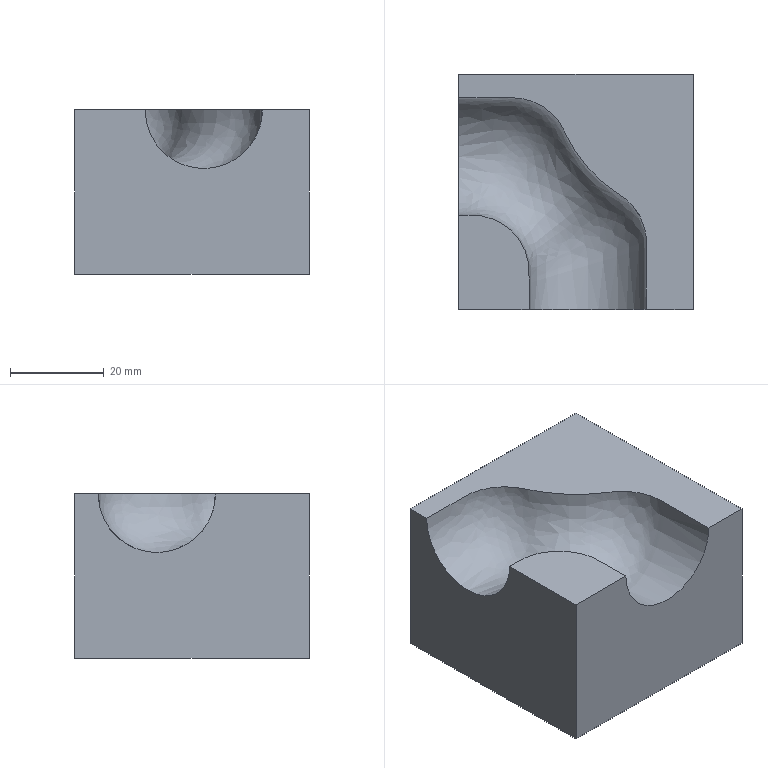NC program | NX | posted with a generic post | part box 50 x 50 x 35 mm
Lines 1 to 1307 of 32931:
N10 G17 G21 G94 G90
(CAVITY_MILL , TOOL : D12)
N12 T00 M6
N14 G54
N16 G17 G0 G90 X-6. Y32.437 S3000 M3
N18 G43 Z10. H0
N20 Z-0.097
N22 G94 G1 Z-0.297 F2500.
N24 X5.4
N26 Y31.532
N28 G2 X14.08 Y28.901 R23.645
N30 X11.92 Y33.111 R41.565
N32 G3 X11.609 Y33.334 R0.377
N34 G1 X9.998 Y33.341
N36 X5.4 Y33.342
N38 Y32.437
N40 X0.
N42 Y26.25
N44 X3.16 Y26.252
N46 G2 X19.984 Y14.699 R18.245
N48 G1 X25.008 Y16.679
N50 G2 X26.652 Y8.373 R23.645
N52 G1 X26.662 Y7.474
N54 X26.663 Y5.4
N56 X28.34
N58 Y14.217
N60 G3 X28.198 Y14.478 R0.312
N62 G2 X26.484 Y15.623 R100.713
N64 X25.008 Y16.679 R41.565
N66 G1 X19.984 Y14.699
N68 G2 X21.252 Y8.298 R18.245
N70 G1 X21.262 Y7.442
N72 X21.264 Y0.591
N74 X21.256 Y0.
N76 X33.748
N78 X33.741 Y0.591
N80 X33.74 Y14.217
N82 G3 X31.151 Y18.999 R5.712
N84 G2 X29.529 Y20.082 R95.313
N86 X16.858 Y35.298 R36.165
N88 G3 X11.724 Y38.733 R5.777
N90 G1 X10.011 Y38.741
N92 X0. Y38.743
N94 Y32.437
N96 X-6.
N98 Z-0.097
N100 G0 Z0.3
N102 Y32.434
N104 Z-0.395
N106 G1 Z-0.595
N108 X5.4
N110 Y31.545
N112 G2 X14.054 Y28.93 R23.661
N114 X12.004 Y32.909 R41.601
N116 G3 X11.822 Y33.205 R3.769
N118 X11.607 Y33.319 R0.261
N120 G1 X5.4 Y33.324
N122 Y32.434
N124 X0.
N126 Y26.261
N128 X3.16 Y26.265
N130 G2 X20.015 Y14.66 R18.261
N132 G1 X25.043 Y16.627
N134 G2 X26.668 Y8.366 R23.661
N136 G1 X26.676 Y7.467
N138 Y5.4
N140 X28.33
N142 Y13.425
N144 X28.327 Y14.197
N146 G3 X28.174 Y14.479 R0.339
N148 G1 X26.712 Y15.443
N150 G2 X25.043 Y16.627 R41.601
N152 G1 X20.015 Y14.66
N154 G2 X21.268 Y8.298 R18.261
N156 G1 X21.276 Y7.442
N158 X21.278 Y0.591
N160 X21.272 Y0.
N162 X33.736
N164 X33.73 Y0.591
N166 Y13.436
N168 X33.727 Y14.22
N170 G3 X31.145 Y18.988 R5.739
N172 G1 X29.708 Y19.935
N174 G2 X16.862 Y35.274 R36.201
N176 G3 X16.287 Y36.242 R9.169
N178 X11.611 Y38.719 R5.661
N180 G1 X0. Y38.728
N182 Y32.434
N184 X-6.
N186 Z-0.395
N188 G0 Z0.003
N190 Z-0.692
N192 G1 Z-0.892
N194 X5.4
N196 Y31.56
N198 G2 X13.994 Y28.981 R23.668
N200 X11.935 Y33. R41.381
N202 G3 X11.767 Y33.244 R0.8
N204 G1 X11.69 Y33.312
N206 X11.588 Y33.305
N208 X5.4 Y33.309
N210 Y32.434
N212 X0.
N214 Y26.282
N216 X3.16 Y26.28
N218 G2 X20.04 Y14.642 R18.268
N220 G1 X25.072 Y16.602
N222 G2 X26.683 Y8.357 R23.668
N224 G1 X26.689 Y7.46
N226 X26.69 Y5.4
N228 X28.315
N230 X28.316 Y13.405
N232 X28.307 Y14.195
N234 G3 X28.153 Y14.479 R0.347
N236 G1 X26.693 Y15.458
N238 G2 X25.072 Y16.602 R41.381
N240 G1 X20.04 Y14.642
N242 G2 X21.284 Y8.298 R18.268
N244 G1 X21.289 Y7.442
N246 X21.292 Y0.591
N248 X21.288 Y0.
N250 X33.72
N252 X33.714 Y0.591
N254 X33.716 Y13.436
N256 X33.706 Y14.258
N258 G3 X31.161 Y18.964 R5.747
N260 G1 X29.701 Y19.943
N262 G2 X16.869 Y35.196 R35.981
N264 G3 X15.149 Y37.458 R6.2
N266 X11.724 Y38.704 R5.846
N268 G1 X0. Y38.713
N270 Y32.434
N272 X-6.
N274 Z-0.692
N276 G0 Z-0.295
N278 Y32.436
N280 Z-0.989
N282 G1 Z-1.189
N284 X5.4
N286 Y31.583
N288 G2 X13.921 Y29.049 R23.678
N290 X11.883 Y33.058 R41.348
N292 G3 X11.573 Y33.28 R0.375
N294 G1 X10.835 Y33.289
N296 X5.4 Y33.288
N298 Y32.436
N300 X0.
N302 Y26.31
N304 X3.16 Y26.316
N306 X3.887 Y26.282
N308 G2 X20.095 Y14.572 R18.278
N310 G1 X25.136 Y16.506
N312 G2 X26.42 Y11.707 R23.678
N314 X26.699 Y8.163 R22.996
N316 G1 X26.703 Y5.4
N318 X28.288
N320 X28.291 Y13.412
N322 X28.283 Y14.218
N324 X28.291 Y14.323
N326 X28.213 Y14.393
N328 X26.709 Y15.4
N330 G2 X25.136 Y16.506 R41.348
N332 G1 X20.095 Y14.572
N334 G2 X21.085 Y10.867 R18.278
N336 X21.299 Y8.155 R17.596
N338 G1 X21.31 Y0.591
N340 X21.305 Y0.
N342 X33.691
N344 X33.687 Y0.591
N346 X33.691 Y13.436
N348 X33.683 Y14.293
N350 G3 X31.42 Y18.745 R5.677
N352 G1 X29.713 Y19.888
N354 G2 X16.822 Y35.24 R35.948
N356 G3 X11.724 Y38.679 R5.775
N358 G1 X10.867 Y38.689
N360 X0.591 Y38.687
N362 X0. Y38.692
N364 Y32.436
N366 X-6.
N368 Z-0.989
N370 G0 Z-0.592
N372 Y32.433
N374 Z-1.287
N376 G1 Z-1.487
N378 X5.4
N380 Y31.62
N382 G2 X13.839 Y29.121 R23.937
N384 X11.854 Y33.065 R41.036
N386 G3 X11.599 Y33.247 R0.307
N388 G1 X10.847 Y33.254
N390 X5.4 Y33.247
N392 Y32.433
N394 X0.
N396 Y26.351
N398 G2 X3.49 Y26.339 R66.439
N400 X16.647 Y20.287 R18.537
N402 X20.169 Y14.496 R18.185
N404 G1 X25.225 Y16.393
N406 G2 X26.726 Y8.333 R23.585
N408 G1 X26.733 Y5.4
N410 X28.258
N412 X28.254 Y14.231
N414 X28.26 Y14.327
N416 X28.178 Y14.376
N418 G3 X27.166 Y15.057 R33.566
N420 G2 X25.225 Y16.393 R41.036
N422 G1 X20.169 Y14.496
N424 G2 X21.326 Y8.298 R18.185
N426 G1 X21.345 Y0.591
N428 X21.341 Y0.
N430 X33.661
N432 X33.654 Y14.234
N434 G3 X31.273 Y18.802 R5.578
N436 X30.098 Y19.591 R38.966
N438 G2 X16.801 Y35.23 R35.636
N440 G3 X11.724 Y38.647 R5.707
N442 G1 X10.867 Y38.654
N444 X1.447 Y38.641
N446 X0. Y38.648
N448 Y32.433
N450 X-6.
N452 Z-1.287
N454 G0 Z-0.889
N456 Z-1.584
N458 G1 Z-1.784
N460 X5.4
N462 Y31.661
N464 G2 X13.742 Y29.214 R24.5
N466 X11.836 Y33.019 R41.039
N468 G3 X11.537 Y33.214 R0.325
N470 G1 X5.4 Y33.204
N472 Y32.433
N474 X0.
N476 Y26.385
N478 G2 X3.16 Y26.397 R111.809
N480 X11.724 Y24.18 R19.1
N482 X20.247 Y14.407 R18.153
N484 G1 X25.316 Y16.268
N486 G2 X26.759 Y8.332 R23.553
N488 G1 X26.771 Y5.4
N490 X28.217
N492 X28.214 Y14.23
N494 X28.224 Y14.311
N496 X28.151 Y14.35
N498 G3 X27.438 Y14.826 R20.331
N500 G2 X25.316 Y16.268 R41.039
N502 G1 X20.247 Y14.407
N504 G2 X21.359 Y8.298 R18.153
N506 G1 X21.391 Y0.591
N508 X21.386 Y0.
N510 X33.618
N512 X33.614 Y14.231
N514 G3 X31.243 Y18.777 R5.547
N516 X30.34 Y19.38 R25.731
N518 G1 X30.277 Y19.42
N520 G2 X16.783 Y35.185 R35.639
N522 G3 X11.528 Y38.614 R5.725
N524 G1 X1.447 Y38.598
N526 X0. Y38.603
N528 Y32.433
N530 X-6.
N532 Z-1.584
N534 G0 Z-1.187
N536 Y32.436
N538 Z-1.881
N540 G1 Z-2.081
N542 X5.4
N544 Y31.71
N546 G2 X13.63 Y29.321 R24.108
N548 X11.814 Y32.976 R40.78
N550 G3 X11.509 Y33.176 R0.332
N552 G1 X5.4 Y33.162
N554 Y32.436
N556 X0.
N558 Y26.428
N560 X3.16 Y26.438
N562 G2 X17.718 Y19.154 R18.708
N564 X20.326 Y14.319 R18.41
N566 G1 X25.408 Y16.145
N568 G2 X26.81 Y8.34 R23.81
N570 G1 X26.823 Y5.4
N572 X28.174
N574 X28.183 Y13.413
N576 X28.175 Y14.206
N578 X28.184 Y14.288
N580 X28.11 Y14.326
N582 X27.592 Y14.677
N584 X27.274 Y14.881
N586 G2 X25.408 Y16.145 R40.78
N588 G1 X20.326 Y14.319
N590 G2 X21.41 Y8.298 R18.41
N592 G1 X21.444 Y0.591
N594 X21.44 Y0.
N596 X33.573
N598 X33.57 Y0.591
N600 X33.583 Y13.436
N602 X33.575 Y14.258
N604 G3 X31.14 Y18.796 R5.547
N606 G1 X30.564 Y19.187
N608 X30.182 Y19.431
N610 G2 X16.765 Y35.133 R35.38
N612 G3 X11.497 Y38.576 R5.732
N614 G1 X1.447 Y38.554
N616 X0. Y38.558
N618 Y32.436
N620 X-6.
N622 Z-1.881
N624 G0 Z-1.484
N626 Y32.435
N628 Z-2.179
N630 G1 Z-2.379
N632 X5.4
N634 Y31.754
N636 G2 X13.496 Y29.448 R24.115
N638 X11.946 Y32.57 R40.388
N640 G1 X11.727 Y33.02
N642 G3 X11.56 Y33.124 R0.185
N644 G1 X5.4 Y33.115
N646 Y32.435
N648 X0.
N650 Y26.48
N652 X3.16 Y26.479
N654 G2 X17.718 Y19.251 R18.715
N656 X20.423 Y14.21 R18.473
N658 G1 X25.519 Y15.995
N660 G2 X26.861 Y8.342 R23.873
N662 G1 X26.877 Y5.4
N664 X28.118
N666 X28.132 Y13.407
N668 X28.122 Y14.212
N670 X28.136 Y14.27
N672 X28.079 Y14.29
N674 X27.603 Y14.605
N676 X27.166 Y14.888
N678 G2 X25.519 Y15.995 R40.388
N680 G1 X20.423 Y14.21
N682 G2 X21.461 Y8.298 R18.473
N684 G1 X21.498 Y1.447
N686 X21.493 Y0.
N688 X33.514
N690 X33.509 Y0.591
N692 X33.532 Y13.436
N694 X33.521 Y14.281
N696 G3 X31.06 Y18.792 R5.495
N698 G1 X30.564 Y19.121
N700 X30.086 Y19.431
N702 G2 X16.844 Y34.846 R34.988
N704 G1 X16.581 Y35.385
N706 G3 X11.553 Y38.524 R5.585
N708 G1 X1.447 Y38.51
N710 X0. Y38.513
N712 Y32.435
N714 X-6.
N716 Z-2.179
N718 G0 Z-1.781
N720 Y32.433
N722 Z-2.476
N724 G1 Z-2.676
N726 X5.4
N728 Y31.806
N730 G2 X13.345 Y29.587 R24.307
N732 X11.727 Y32.92 R40.275
N734 G3 X11.504 Y33.066 R0.243
N736 G1 X5.4 Y33.059
N738 Y32.433
N740 X0.
N742 Y26.549
N744 G2 X3.368 Y26.527 R100.562
N746 X16.862 Y20.406 R18.907
N748 X20.53 Y14.087 R18.513
N750 G1 X25.643 Y15.823
N752 G2 X26.912 Y8.335 R23.913
N754 G1 X26.926 Y5.4
N756 X28.054
N758 X28.07 Y13.411
N760 X28.061 Y14.211
N762 X28.076 Y14.243
N764 X28.041 Y14.249
N766 X27.645 Y14.511
N768 X27.079 Y14.863
N770 G2 X25.643 Y15.823 R40.275
N772 G1 X20.53 Y14.087
N774 G2 X21.512 Y8.298 R18.513
N776 G1 X21.55 Y0.591
N778 X21.548 Y0.
N780 X33.448
N782 X33.444 Y0.591
N784 X33.47 Y13.436
N786 X33.461 Y14.272
N788 G3 X31.023 Y18.75 R5.445
N790 G1 X30.564 Y19.055
N792 X29.96 Y19.431
N794 G2 X16.689 Y35.052 R34.875
N796 G3 X11.498 Y38.466 R5.643
N798 G1 X0.591 Y38.453
N800 X0. Y38.457
N802 Y32.433
N804 X-6.
N806 Z-2.476
N808 G0 Z-2.079
N810 Y32.434
N812 Z-2.773
N814 G1 Z-2.973
N816 X5.4
N818 Y31.879
N820 G2 X13.196 Y29.73 R24.609
N822 X11.669 Y32.904 R40.408
N824 G1 X11.629 Y32.996
N826 X11.53
N828 X5.4 Y32.989
N830 Y32.434
N832 X0.
N834 Y26.617
N836 X0.01
N838 X3.16 Y26.609
N840 G2 X16.006 Y21.397 R19.209
N842 X20.646 Y13.974 R17.982
N844 G1 X25.784 Y15.636
N846 G2 X26.695 Y11.67 R23.382
N848 X26.963 Y8.313 R21.11
N850 G1 X26.98 Y5.4
N852 X27.991
N854 X28.009 Y13.416
N856 X28.002 Y14.175
N858 X28.008 Y14.242
N860 X27.944 Y14.262
N862 X27.842 Y14.318
N864 X26.971 Y14.852
N866 G2 X25.784 Y15.636 R39.985
N868 G1 X20.646 Y13.974
N870 G2 X21.355 Y10.867 R17.982
N872 X21.563 Y8.298 R15.71
N874 G1 X21.613 Y0.02
N876 Y0.
N878 X33.383
N880 X33.38 Y0.591
N882 X33.409 Y13.436
N884 X33.401 Y14.293
N886 G3 X30.564 Y18.983 R5.513
N888 G1 X29.833 Y19.431
N890 G2 X22.745 Y25.426 R34.585
N892 G1 X22.023 Y26.282
N894 G2 X16.632 Y35.031 R35.008
N896 G3 X11.524 Y38.396 R5.551
N898 G1 X0. Y38.384
N900 Y32.434
N902 X-6.
N904 Z-2.773
N906 G0 Z-2.376
N908 Z-3.071
N910 G1 Z-3.271
N912 X5.4
N914 Y31.952
N916 G2 X13.019 Y29.895 R24.659
N918 X11.626 Y32.851 R39.555
N920 G1 X11.598 Y32.93
N922 X11.515 Y32.925
N924 X5.4 Y32.916
N926 Y32.434
N928 X0.
N930 Y26.689
N932 X3.16 Y26.681
N934 G2 X16.862 Y20.652 R19.259
N936 X20.783 Y13.822 R18.257
N938 G1 X25.936 Y15.438
N940 G2 X26.998 Y9.37 R23.657
N942 G1 X27.033 Y8.419
N944 X27.058 Y5.4
N946 X27.92
N948 X27.938 Y14.148
N950 X27.948 Y14.193
N952 X27.902 Y14.194
N954 X27.848 Y14.225
N956 G2 X25.936 Y15.438 R39.555
N958 G1 X20.783 Y13.822
N960 G2 X21.602 Y9.155 R18.257
N962 G1 X21.633 Y8.298
N964 X21.697 Y0.591
N966 X21.695 Y0.
N968 X33.31
N970 Y0.002
N972 X33.338 Y14.293
N974 G3 X30.564 Y18.892 R5.477
N976 G2 X16.602 Y34.949 R34.155
N978 G3 X11.507 Y38.325 R5.521
N980 G1 X0. Y38.309
N982 Y32.434
N984 X-6.
N986 Z-3.071
N988 G0 Z-2.673
N990 Y32.435 Z-3.368
N992 G1 Z-3.568
N994 X5.4
N996 Y32.036
N998 G2 X12.829 Y30.069 R24.969
N1000 X11.562 Y32.8 R39.199
N1002 G1 X11.551 Y32.859
N1004 X11.492 Y32.847
N1006 X5.4 Y32.833
N1008 Y32.435
N1010 X0.
N1012 Y26.781
N1014 X3.16 Y26.769
N1016 G2 X15.605 Y22. R19.569
N1018 X20.912 Y13.708 R17.587
N1020 G1 X26.093 Y15.23
N1022 G2 X26.491 Y13.679 R22.987
N1024 G1 X26.691 Y12.643
N1026 G2 X27.099 Y8.814 R22.848
N1028 G1 X27.108 Y8.381
N1030 X27.134 Y5.4
N1032 X27.835
N1034 X27.855 Y14.13
N1036 X27.846 Y14.135
N1038 G2 X26.093 Y15.23 R39.199
N1040 G1 X20.912 Y13.708
N1042 G2 X21.203 Y12.58 R17.587
N1044 G1 X21.388 Y11.621
N1046 G2 X21.7 Y8.696 R17.448
N1048 G1 X21.709 Y8.298
N1050 X21.776 Y0.591
N1052 X21.774 Y0.
N1054 X33.222
N1056 Y0.006
N1058 X33.255 Y14.293
N1060 G3 X30.564 Y18.802 R5.374
N1062 G2 X16.544 Y34.883 R33.799
N1064 G3 X11.48 Y38.247 R5.476
N1066 G1 X0.007 Y38.22
N1068 X0.
N1070 Y32.435
N1072 X-6.
N1074 Z-3.368
N1076 G0 Z-2.971
N1078 Y32.432
N1080 Z-3.665
N1082 G1 Z-3.865
N1084 X5.4
N1086 Y32.133
N1088 G2 X12.636 Y30.252 R25.239
N1090 X11.498 Y32.749 R38.881
N1092 G1 X5.4 Y32.732
N1094 Y32.432
N1096 X0.
N1098 Y26.882
N1100 X0.032
N1102 X3.16 Y26.869
N1104 G2 X16.006 Y21.785 R19.839
N1106 X20.842 Y14.293 R17.777
N1108 X21.044 Y13.594 R22.457
N1110 G1 X26.256 Y15.004
N1112 G2 X27.176 Y9.356 R27.857
N1114 G1 X27.219 Y5.4
N1116 X27.749
N1118 X27.772 Y14.069
N1120 G2 X26.256 Y15.004 R38.881
N1122 G1 X21.044 Y13.594
N1124 G2 X21.777 Y9.155 R22.457
N1126 G1 X21.872 Y0.591
N1128 X21.87 Y0.
N1130 X33.135
N1132 X33.172 Y14.106
N1134 G3 X30.54 Y18.706 R5.31
N1136 G2 X16.482 Y34.828 R33.481
N1138 G3 X11.502 Y38.149 R5.372
N1140 G1 X0.047 Y38.118
N1142 X0.
N1144 Y32.432
N1146 X-6.
N1148 Z-3.665
N1150 G0 Z-3.268
N1152 Y32.43
N1154 Z-3.963
N1156 G1 Z-4.163
N1158 X5.4
N1160 Y32.229
N1162 G2 X12.439 Y30.44 R25.453
N1164 X11.438 Y32.65 R35.685
N1166 G1 X5.4 Y32.632
N1168 Y32.43
N1170 X0.
N1172 Y26.982
N1174 X0.038
N1176 X2.802 Y26.971
N1178 G2 X15.932 Y22. R20.053
N1180 X20.64 Y15.149 R17.441
N1182 G1 X20.956 Y14.293
N1184 G3 X21.153 Y13.54 R20.986
N1186 G1 X21.202 Y13.362
N1188 X26.413 Y14.776
N1190 G2 X27.27 Y8.689 R24.635
N1192 G1 X27.3 Y6.657
N1194 X27.315 Y5.4
N1196 X27.637
N1198 X27.676 Y14.01
N1200 G2 X26.413 Y14.776 R38.182
N1202 G1 X21.202 Y13.362
N1204 G2 X21.871 Y8.609 R19.235
N1206 G1 X21.901 Y6.585
N1208 X21.971 Y0.591
N1210 X21.969 Y0.
N1212 X33.019
N1214 X33.015 Y0.591
N1216 X33.077 Y14.293
N1218 G3 X30.564 Y18.578 R5.215
N1220 G2 X17.718 Y31.983 R32.782
N1222 X16.402 Y34.777 R30.285
N1224 G3 X11.504 Y38.05 R5.276
N1226 G1 X0.035 Y38.015
N1228 X0.
N1230 Y32.43
N1232 X-6.
N1234 Z-3.963
N1236 G0 Z-3.565
N1238 Y32.434
N1240 Z-4.26
N1242 G1 Z-4.46
N1244 X5.4
N1246 Y32.337
N1248 G2 X12.24 Y30.633 R25.834
N1250 X12. Y31.154 R37.747
N1252 X11.359 Y32.552 R16.799
N1254 G1 X5.4 Y32.531
N1256 Y32.434
N1258 X0.
N1260 Y27.087
N1262 G2 X4.016 Y27.039 R100.894
N1264 X16.006 Y22.102 R20.434
N1266 X21.144 Y14.005 R17.208
N1268 X21.359 Y13.215 R20.272
N1270 G1 X26.597 Y14.531
N1272 G2 X27.37 Y8.348 R25.672
N1274 G1 X27.419 Y5.4
N1276 X27.529
N1278 X27.571 Y12.595
N1280 X27.57 Y13.95
N1282 G2 X26.597 Y14.531 R37.747
N1284 G1 X21.359 Y13.215
N1286 G2 X21.97 Y8.298 R20.272
N1288 G1 X22.083 Y1.447
N1290 X22.085 Y0.
N1292 X32.905
N1294 X32.902 Y0.591
N1296 X32.971 Y12.58
N1298 X32.97 Y14.114
N1300 G3 X30.388 Y18.559 R5.12
N1302 G2 X16.862 Y33.511 R32.347
N1304 X16.315 Y34.701 R11.399
N1306 G3 X11.532 Y37.952 R5.117
N1308 G1 X0.021 Y37.913
N1310 X0.
N1312 Y32.434
N1314 X-6.
N1316 Z-4.26
N1318 G0 Z-3.863
N1320 Y32.439
N1322 Z-4.557
N1324 G1 Z-4.757
N1326 X8.453
N1328 X5.612 Y32.426
N1330 G2 X12.007 Y30.849 R26.017
N1332 X11.293 Y32.453 R46.023
N1334 G1 X8.453 Y32.439
N1336 X8.427 Y37.839
N1338 X0.021 Y37.8
N1340 X0.
N1342 Y27.201
N1344 X2.304 Y27.193
N1346 X3.16 Y27.18
N1348 X4.016 Y27.14
N1350 X4.873 Y27.075
N1352 G2 X16.317 Y22. R20.617
N1354 X21.429 Y13.434 R17.103
N1356 X21.512 Y13.084 R22.186
N1358 G1 X26.775 Y14.293
N1360 G2 X27.443 Y9.455 R27.586
N1362 G1 X27.462 Y12.598
N1364 X27.463 Y13.872
N1366 X26.867 Y14.235
N1368 X26.775 Y14.293
N1370 X21.512 Y13.084
N1372 G2 X22.066 Y8.769 R22.186
N1374 X22.209 Y0. R333.954
N1376 G1 X32.791
N1378 X32.788 Y0.591
N1380 X32.862 Y12.58
N1382 X32.863 Y14.109
N1384 G3 X30.479 Y18.358 R4.974
N1386 G1 X29.708 Y18.828
N1388 X28.851 Y19.365
N1390 G2 X18.219 Y30.564 R31.327
N1392 X16.191 Y34.736 R40.623
N1394 G3 X11.487 Y37.854 R5.071
N1396 G1 X8.427 Y37.839
N1398 X8.455 Y31.839
N1400 X-6.
N1402 Z-4.557
N1404 G0 Z-4.16
N1406 Y32.31
N1408 Z-4.854
N1410 G1 Z-5.054
N1412 X9.253
N1414 G2 X7.281 Y32.297 R2116.254
N1416 X11.768 Y31.067 R26.478
N1418 X11.225 Y32.325 R40.424
N1420 X9.253 Y32.31 R2116.254
N1422 G1 X9.215 Y37.709
N1424 G2 X0.021 Y37.664 R2110.854
N1426 G1 X0.
N1428 Y27.337
N1430 X0.591 Y27.339
N1432 X2.304 Y27.327
N1434 X3.16 Y27.313
N1436 G2 X15.149 Y23.145 R21.078
N1438 X21.551 Y13.436 R16.917
N1440 X21.677 Y12.89 R22.788
N1442 G1 X26.953 Y14.041
N1444 G2 X27.348 Y11.801 R28.188
N1446 G1 X27.354 Y12.603
N1448 X27.355 Y13.808
N1450 G2 X26.953 Y14.041 R38.096
N1452 G1 X21.677 Y12.89
N1454 G2 X22.173 Y9.155 R22.788
N1456 G1 X22.195 Y8.298
N1458 G2 X22.333 Y0. R328.257
N1460 G1 X32.67
N1462 X32.667 Y0.591
N1464 X32.754 Y12.58
N1466 X32.756 Y14.039
N1468 G3 X30.207 Y18.399 R4.994
N1470 G2 X22.342 Y24.569 R32.696
N1472 G1 X21.144 Y25.979
N1474 G2 X16.119 Y34.625 R35.024
N1476 G3 X11.483 Y37.727 R4.954
N1478 G2 X9.215 Y37.709 R2110.854
N1480 G1 X9.257 Y31.71
N1482 Z-4.854
N1484 G0 Z-4.457
N1486 X-6. Y32.182
N1488 Z-5.152
N1490 G1 Z-5.352
N1492 X9.834
N1494 G2 X8.515 Y32.172 R1814.426
N1496 X11.538 Y31.285 R27.11
N1498 X11.153 Y32.194 R42.32
N1500 X9.834 Y32.182 R1814.426
N1502 G1 X9.79 Y37.582
N1504 G2 X0.023 Y37.53 R1809.026
N1506 G1 X0. Y37.529
N1508 Y27.472
N1510 X0.591 Y27.473
N1512 G2 X4.016 Y27.41 R72.624
N1514 X15.785 Y22.857 R21.71
N1516 X21.699 Y13.436 R16.784
N1518 X21.855 Y12.716 R23.51
N1520 G1 X27.15 Y13.776
N1522 G2 X27.24 Y13.304 R28.91
N1524 G1 X27.247 Y13.722
N1526 X27.15 Y13.776
N1528 X21.855 Y12.716
N1530 G2 X22.311 Y8.298 R23.51
N1532 G1 X22.327 Y7.442
N1534 X22.414 Y4.015
N1536 G2 X22.466 Y0. R160.544
N1538 G1 X32.528
N1540 G2 X32.652 Y13.92 R741.705
N1542 G3 X30.867 Y17.774 R4.862
N1544 X29.929 Y18.409 R6.303
N1546 G2 X18.379 Y29.708 R30.375
N1548 X16.035 Y34.525 R36.92
N1550 G3 X11.456 Y37.596 R4.884
N1552 G2 X9.79 Y37.582 R1809.026
N1554 G1 X9.839 Y31.582
N1556 Z-5.152
N1558 G0 Z-4.754
N1560 X-6. Y32.055
N1562 Z-5.449
N1564 G1 Z-5.649
N1566 X10.321
N1568 G2 X9.563 Y32.049 R1785.358
N1570 X11.309 Y31.509 R27.847
N1572 X11.079 Y32.062 R46.115
N1574 X10.321 Y32.055 R1785.358
N1576 G1 X10.271 Y37.455
N1578 G2 X0.013 Y37.39 R1779.958
N1580 G1 X0.
N1582 Y27.614
N1584 X0.591 Y27.615
N1586 G2 X4.873 Y27.476 R48.318
N1588 X15.149 Y23.538 R22.447
N1590 X21.643 Y14.281 R16.597
N1592 X22.417 Y8.846 R22.445
N1594 G1 X22.427 Y8.298
N1596 G2 X22.617 Y0.041 R233.449
N1598 G1 Y0.
N1600 X32.384
N1602 G2 X32.507 Y13.436 R708.625
N1604 G1 X32.5 Y14.12
N1606 G3 X30.332 Y17.976 R4.595
N1608 G1 X29.708 Y18.364
N1610 X29.328 Y18.575
N1612 G2 X17.288 Y31.42 R29.847
N1614 X15.945 Y34.435 R40.715
N1616 G3 X11.429 Y37.466 R4.809
N1618 G2 X10.271 Y37.455 R1779.958
N1620 G1 X10.327 Y31.455
N1622 Z-5.449
N1624 G0 Z-5.052
N1626 X-6. Y31.928
N1628 Z-5.746
N1630 G1 Z-5.946
N1632 X10.762
N1634 X10.528 Y31.923
N1636 G2 X11.071 Y31.75 R28.049
N1638 G1 X11.019 Y31.881
N1640 X10.995 Y31.933
N1642 X10.762 Y31.928
N1644 X10.65 Y37.327
N1646 X10.418 Y37.322
N1648 G2 X0. Y37.224 R480.775
N1650 G1 Y27.778
N1652 G2 X4.016 Y27.701 R77.359
N1654 X14.293 Y24.309 R22.649
N1656 G1 X15.149 Y23.751
N1658 X16.006 Y23.152
N1660 X16.363 Y22.857
N1662 X16.862 Y22.388
N1664 X17.29 Y22.
N1666 G2 X21.277 Y16.006 R16.351
N1668 X22.553 Y9.155 R23.688
N1670 G1 X22.573 Y8.298
N1672 X22.596 Y7.442
N1674 X22.66 Y5.729
N1676 G2 X22.772 Y0. R134.06
N1678 G1 X32.233
N1680 G2 X32.371 Y13.436 R716.302
N1682 G1 X32.366 Y14.005
N1684 G3 X29.86 Y18.115 R4.695
N1686 G2 X17.53 Y30.564 R29.16
N1688 G1 X17.111 Y31.42
N1690 G2 X15.994 Y33.989 R30.763
N1692 G1 X15.713 Y34.594
N1694 G3 X11.305 Y37.341 R4.744
N1696 G2 X10.65 Y37.327 R480.775
N1698 G1 X10.774 Y31.328
N1700 Z-5.746
N1702 G0 Z-5.349
N1704 X-6. Y32.5
N1706 Z-6.044
N1708 G1 Z-6.244
N1710 X0.
N1712 Y27.941
N1714 G2 X4.873 Y27.794 R57.34
N1716 X14.293 Y24.516 R23.749
N1718 G1 X14.677 Y24.281
N1720 G2 X22.186 Y13.423 R16.3
N1722 X22.71 Y8.617 R30.395
N1724 G1 X22.744 Y7.442
N1726 X22.812 Y5.729
N1728 G2 X22.938 Y0. R126.059
N1730 G1 X32.058
N1732 G2 X32.235 Y13.784 R531.817
N1734 G3 X29.749 Y17.987 R4.597
N1736 G2 X16.952 Y31.38 R28.473
N1738 G1 X16.933 Y31.42
N1740 X16.862 Y31.567
N1742 G2 X15.772 Y34.145 R35.379
N1744 G3 X11.269 Y37.184 R4.697
N1746 G2 X0. Y37.059 R473.678
N1748 G1 Y32.5
N1750 X-6.
N1752 Z-6.044
N1754 G0 Z-5.646
N1756 Z-6.341
N1758 G1 Z-6.541
N1760 X0.
N1762 Y28.121
N1764 G2 X4.873 Y27.963 R56.613
N1766 X14.293 Y24.749 R24.54
N1768 G1 X14.775 Y24.458
N1770 G2 X22.276 Y13.87 R16.17
N1772 X22.857 Y8.638 R27.741
N1774 G1 X22.866 Y8.298
N1776 G2 X23.12 Y0.046 R161.753
N1778 G1 Y0.
N1780 X31.883
N1782 G2 X32.071 Y13.805 R523.089
N1784 G3 X29.665 Y17.834 R4.382
N1786 G2 X16.862 Y31.15 R27.887
N1788 X15.644 Y34.052 R42.12
N1790 G3 X11.218 Y37.029 R4.598
N1792 G2 X0. Y36.88 R413.742
N1794 G1 Y32.5
N1796 X-6.
N1798 Z-6.341
N1800 G0 Z-5.944
N1802 Z-6.638
N1804 G1 Z-6.838
N1806 X0.
N1808 Y28.312
N1810 G2 X4.873 Y28.163 R62.585
N1812 X16.006 Y23.917 R25.875
N1814 X22.556 Y13.436 R16.049
N1816 X23.013 Y9.155 R31.205
N1818 G1 X23.038 Y8.298
N1820 G2 X23.305 Y0.591 R177.807
N1822 G1 X23.306 Y0.014
N1824 Y0.
N1826 X31.689
N1828 Y0.024
N1830 G2 X31.906 Y13.748 R482.698
N1832 G3 X29.529 Y17.699 R4.263
N1834 G2 X18.828 Y27.138 R27.237
N1836 X15.492 Y33.989 R33.768
N1838 G3 X11.724 Y36.833 R4.446
N1840 G1 X10.867 Y36.841
N1842 G2 X0. Y36.689 R351.124
N1844 G1 Y32.5
N1846 X-6.
N1848 Z-6.638
N1850 G0 Z-6.241
N1852 Z-6.936
N1854 G1 Z-7.136
N1856 X0.
N1858 Y28.512
N1860 G2 X4.873 Y28.371 R76.427
N1862 X15.431 Y24.569 R27.375
N1864 X22.606 Y14.293 R15.775
N1866 X23.21 Y8.298 R32.069
N1868 X23.513 Y0.591 R158.912
N1870 G1 X23.514 Y0.
N1872 X31.488
N1874 G2 X31.726 Y13.752 R424.391
N1876 G3 X29.614 Y17.408 R3.992
N1878 G2 X27.428 Y18.621 R74.594
N1880 X17.904 Y28.224 R25.705
N1882 X15.357 Y33.823 R34.974
N1884 G3 X11.193 Y36.668 R4.266
N1886 G2 X0.081 Y36.487 R333.945
N1888 G1 X0.
N1890 Y32.5
N1892 X-6.
N1894 Z-6.936
N1896 G0 Z-6.538
N1898 Z-7.233
N1900 G1 Z-7.433
N1902 X0.
N1904 Y28.728
N1906 X0.591 Y28.727
N1908 G2 X4.873 Y28.579 R62.646
N1910 X15.775 Y24.643 R28.559
N1912 X22.693 Y14.89 R15.244
N1914 X23.397 Y8.298 R30.896
N1916 X23.724 Y0. R130.358
N1918 G1 X31.26
N1920 X31.258 Y0.185
N1922 G2 X31.538 Y13.745 R427.789
N1924 G3 X29.51 Y17.224 R3.764
N1926 G2 X25.688 Y19.431 R48.817
N1928 X17.744 Y27.995 R24.131
N1930 X15.214 Y33.688 R35.476
N1932 G3 X11.151 Y36.467 R4.119
N1934 G2 X0. Y36.256 R259.921
N1936 G1 Y32.5
N1938 X-6.
N1940 Z-7.233
N1942 G0 Z-6.836
N1944 Z-7.53
N1946 G1 Z-7.73
N1948 X0.
N1950 Y28.963
N1952 X1.53 Y28.959
N1954 G2 X6.585 Y28.521 R30.27
N1956 X15.617 Y25.052 R31.902
N1958 X23.01 Y14.607 R15.154
N1960 X23.596 Y8.298 R36.297
N1962 X23.97 Y0.591 R133.209
N1964 G1 X23.972 Y0.
N1966 X31.023
N1968 Y0.052
N1970 G2 X31.33 Y13.61 R323.904
N1972 G3 X29.105 Y17.225 R3.785
N1974 G2 X19.645 Y24.569 R25.591
N1976 X15.149 Y33.355 R29.486
N1978 G3 X13.436 Y35.642 R4.43
N1980 X11.295 Y36.254 R3.524
N1982 G2 X0.591 Y36.025 R244.524
N1984 G1 X0.
N1986 Y32.5
N1988 X-6.
N1990 Z-7.53
N1992 G0 Z-7.133
N1994 Z-7.828
N1996 G1 Z-8.028
N1998 X0.
N2000 Y29.22
N2002 X1.938 Y29.214
N2004 G2 X8.577 Y28.258 R24.026
N2006 X15.538 Y25.426 R36.417
N2008 X23.325 Y14.293 R15.019
N2010 X23.812 Y8.298 R50.651
N2012 X24.217 Y0.591 R101.893
N2014 G1 X24.22 Y0.
N2016 X30.783
N2018 G2 X31.104 Y13.604 R289.404
N2020 G3 X28.966 Y17.036 R3.558
N2022 G2 X19.904 Y23.713 R25.128
N2024 X15.005 Y33.133 R29.192
N2026 G3 X11.724 Y36.003 R3.888
N2028 G1 X10.867 Y36.015
N2030 G2 X0. Y35.794 R235.781
N2032 G1 Y32.5
N2034 X-6.
N2036 Z-7.828
N2038 G0 Z-7.43
N2040 Z-8.125
N2042 G1 Z-8.325
N2044 X0.
N2046 Y29.477
N2048 X1.533 Y29.472
N2050 G2 X5.729 Y29.158 R29.661
N2052 X16.006 Y25.515 R36.743
N2054 X23.584 Y14.293 R14.688
N2056 X24.051 Y8.298 R62.837
N2058 X24.468 Y0. R93.635
N2060 G1 X30.537
N2062 Y0.108
N2064 G2 X30.878 Y13.59 R323.277
N2066 G3 X28.795 Y16.85 R3.355
N2068 G2 X18.793 Y24.569 R23.722
N2070 X14.777 Y33.129 R29.958
N2072 G3 X11.034 Y35.803 R3.702
N2074 G2 X0.02 Y35.531 R217.929
N2076 G1 X0.
N2078 Y32.5
N2080 X-6.
N2082 Z-8.125
N2084 G0 Z10.
N2086 X27.496 Y-6.
N2088 Z-8.422
N2090 G1 Z-8.622
N2092 Y0.
N2094 X30.244
N2096 Y0.057
N2098 Y0.591
N2100 G2 X30.645 Y13.436 R285.528
N2102 G3 X28.851 Y16.512 R3.092
N2104 G2 X21.643 Y20.838 R27.015
N2106 X23.869 Y14.293 R15.32
N2108 X24.291 Y8.298 R74.941
N2110 X24.747 Y0.111 R96.264
N2112 G1 Y0.
N2114 X27.496
N2116 Y-6.
N2118 Z-8.422
N2120 G0 Z-8.025
N2122 Z-8.72
N2124 G1 Z-8.92
N2126 Y0.
N2128 X29.946
N2130 Y0.077
N2132 G2 X30.391 Y13.517 R238.563
N2134 G3 X28.648 Y16.282 R2.798
N2136 G2 X22.925 Y19.311 R31.724
N2138 X24.18 Y14.293 R16.167
N2140 G1 X24.251 Y13.436
N2142 X24.53 Y8.298
N2144 G2 X25.055 Y0. R73.679
N2146 G1 X27.496
N2148 Y-6.
N2150 Z-8.72
N2152 G0 Z-8.322
N2154 Z-9.017
N2156 G1 Z-9.217
N2158 Y0.
N2160 X29.64
N2162 G2 X29.638 Y0.215 R7.503
N2164 X30.113 Y13.513 R248.598
N2166 G3 X28.466 Y16.057 R2.548
N2168 G2 X23.801 Y18.233 R33.526
N2170 X24.482 Y14.411 R16.093
N2172 G1 X24.822 Y8.298
N2174 X24.918 Y7.442
N2176 G2 X25.354 Y0.591 R66.012
N2178 G1 X25.359 Y0.
N2180 X27.496
N2182 Y-6.
N2184 Z-9.017
N2186 G0 Z-8.62
N2188 Z-9.314
N2190 G1 Z-9.514
N2192 Y0.
N2194 X29.283
N2196 X29.285 Y0.591
N2198 G2 X29.828 Y13.41 R224.778
N2200 G3 X28.223 Y15.831 R2.38
N2202 G2 X24.488 Y17.354 R34.58
N2204 X24.859 Y13.821 R20.574
N2206 G3 X25.426 Y5.397 R86.492
N2208 G2 X25.708 Y0.015 R47.136
N2210 G1 Y0.
N2212 X27.496
N2214 Y-6.
N2216 Z-9.314
N2218 G0 Z-8.917
N2220 Z-9.612
N2222 G1 Z-9.812
N2224 Y0.
N2226 X28.923
N2228 Y0.088
N2230 G2 X29.512 Y13.341 R181.052
N2232 G3 X28.121 Y15.49 R2.1
N2234 G1 X25.426 Y16.447
N2236 X25.073 Y16.597
N2238 X25.209 Y14.293
N2240 X25.204 Y13.436
N2242 X25.343 Y9.155
N2244 X25.427 Y8.298
N2246 G2 X26.078 Y0.05 R53.092
N2248 G1 Y0.
N2250 X27.496
N2252 Y-6.
N2254 Z-9.612
N2256 G0 Z-9.214
N2258 Z-9.909
N2260 G1 Z-10.109
N2262 Y0.
N2264 X28.514
N2266 X28.517 Y0.591
N2268 G2 X29.185 Y13.436 R186.683
N2270 G3 X27.995 Y15.16 R1.766
N2272 G1 X25.64 Y15.87
N2274 G3 X25.685 Y9.155 R57.758
N2276 G2 X26.482 Y0.166 R63.473
N2278 G1 X26.483 Y0.
N2280 X27.496
N2282 Y-6.
N2284 Z-9.909
N2286 G0 Z-9.512
N2288 Y-6.206
N2290 Z-10.206
N2292 G1 Z-10.406
N2294 Y0.
N2296 X28.088
N2298 Y0.061
N2300 G2 X28.857 Y13.195 R121.
N2302 G3 X27.723 Y14.831 R1.511
N2304 G1 X26.095 Y15.239
N2306 G3 X26.334 Y7.143 R30.008
N2308 G2 X26.911 Y0.591 R42.756
N2310 G1 X26.916 Y0.
N2312 X27.496
N2314 Y-6.206
N2316 Z-10.206
N2318 G0 Z-9.809
N2320 Y-6.695
N2322 Z-10.504
N2324 G1 Z-10.704
N2326 Y0.
N2328 X27.613
N2330 G2 X28.462 Y13.259 R118.291
N2332 G3 X27.709 Y14.346 R0.996
N2334 G1 X26.544 Y14.629
N2336 G3 X26.59 Y8.399 R17.56
N2338 G2 X27.382 Y0.591 R46.43
N2340 G1 X27.389 Y0.
N2342 X27.496
N2344 Y-6.695
N2346 Z-10.504
N2348 G0 Z10.
N2350 X-6. Y32.495
N2352 Z-8.422
N2354 G1 Z-8.622
N2356 X0.
N2358 Y29.745
N2360 G2 X5.729 Y29.427 R42.515
N2362 X13.211 Y27.138 R37.607
N2364 G1 X14.293 Y26.703
N2366 G2 X18.533 Y24.282 R18.429
N2368 X14.546 Y33.03 R30.828
N2370 G3 X11.012 Y35.554 R3.455
N2372 G2 X0. Y35.244 R174.979
N2374 G1 Y32.495
N2376 X-6.
N2378 Z-8.422
N2380 G0 Z-8.025
N2382 Z-8.72
N2384 G1 Z-8.92
N2386 X0.
N2388 Y30.054
N2390 X1.737 Y30.044
N2392 G2 X8.374 Y29.094 R24.571
N2394 X14.293 Y27.042 R57.359
N2396 G1 X15.149 Y26.72
N2398 G2 X17.157 Y25.701 R49.199
N2400 X14.53 Y32.277 R30.804
N2402 G3 X13.951 Y33.724 R5.6
N2404 X11.051 Y35.285 R3.116
N2406 G2 X0.591 Y34.96 R164.515
N2408 G1 X0. Y34.959
N2410 Y32.495
N2412 X-6.
N2414 Z-8.72
N2416 G0 Z-8.322
N2418 Z-9.017
N2420 G1 Z-9.217
N2422 X0.
N2424 Y30.367
N2426 X1.615 Y30.358
N2428 G2 X9.691 Y29.002 R25.629
N2430 G1 X13.381 Y27.751
N2432 G2 X16.192 Y26.645 R31.491
N2434 X14.263 Y32.277 R34.343
N2436 G3 X13.284 Y34.141 R3.969
N2438 X11.061 Y35.016 R2.781
N2440 G2 X0.032 Y34.636 R159.084
N2442 G1 X0.
N2444 Y32.495
N2446 X-6.
N2448 Z-9.017
N2450 G0 Z-8.62
N2452 Z-9.314
N2454 G1 Z-9.514
N2456 X0.
N2458 Y30.683
N2460 G2 X7.442 Y29.974 R27.603
N2462 X15.412 Y27.413 R139.377
N2464 X13.953 Y32.277 R43.52
N2466 G3 X13.14 Y33.852 R3.541
N2468 X10.969 Y34.716 R2.619
N2470 G2 X0.591 Y34.29 R122.092
N2472 G1 X0. Y34.289
N2474 Y32.495
N2476 X-6.
N2478 Z-9.314
N2480 G0 Z-8.917
N2482 Z-9.612
N2484 G1 Z-9.812
N2486 X0.
N2488 Y31.081
N2490 X1.602 Y31.071
N2492 G2 X8.601 Y29.988 R24.093
N2494 G1 X14.711 Y28.091
N2496 X14.486 Y28.851
N2498 X13.643 Y32.277
N2500 X13.436 Y32.834
N2502 G3 X10.867 Y34.381 R2.492
N2504 G2 X0. Y33.936 R118.254
N2506 G1 Y32.495
N2508 X-6.
N2510 Z-9.612
N2512 G0 Z-9.214
N2514 Z-9.909
N2516 G1 Z-10.109
N2518 X0.
N2520 Y31.466
N2522 X1.821 Y31.454
N2524 G2 X8.099 Y30.507 R22.222
N2526 G1 X14.066 Y28.706
N2528 X13.436 Y31.768
N2530 X13.304 Y32.277
N2532 G3 X10.734 Y34.068 R2.402
N2534 G2 X0.591 Y33.52 R106.051
N2536 G1 X0. Y33.517
N2538 Y32.495
N2540 X-6.
N2542 Z-9.909
N2544 G0 Z-9.512
N2546 X-6.202
N2548 Z-10.206
N2550 G1 Z-10.406
N2552 X0.
N2554 Y31.922
N2556 X1.68 Y31.907
N2558 G2 X8.623 Y30.743 R22.422
N2560 G1 X9.156 Y30.564
N2562 X13.485 Y29.306
N2564 G3 X12.91 Y32.277 R22.602
N2566 X10.867 Y33.678 R1.919
N2568 G2 X0. Y33.1 R94.982
N2570 G1 Y32.495
N2572 X-6.202
N2574 Z-10.206
N2576 G0 Z-9.809
N2578 X-6.703
N2580 Z-10.504
N2582 G1 Z-10.704
N2584 X0.
N2586 Y32.386
N2588 X1.886 Y32.366
N2590 G2 X7.444 Y31.525 R20.225
N2592 G1 X12.58 Y29.995
N2594 X12.925 Y29.913
N2596 G3 X12.58 Y32.102 R11.627
N2598 X10.867 Y33.287 R1.611
N2600 G2 X0.591 Y32.61 R82.321
N2602 G1 X0. Y32.605
N2604 Y32.495
N2606 X-6.703
N2608 Z-10.504
N2610 G0 Z10.
N2612 M5